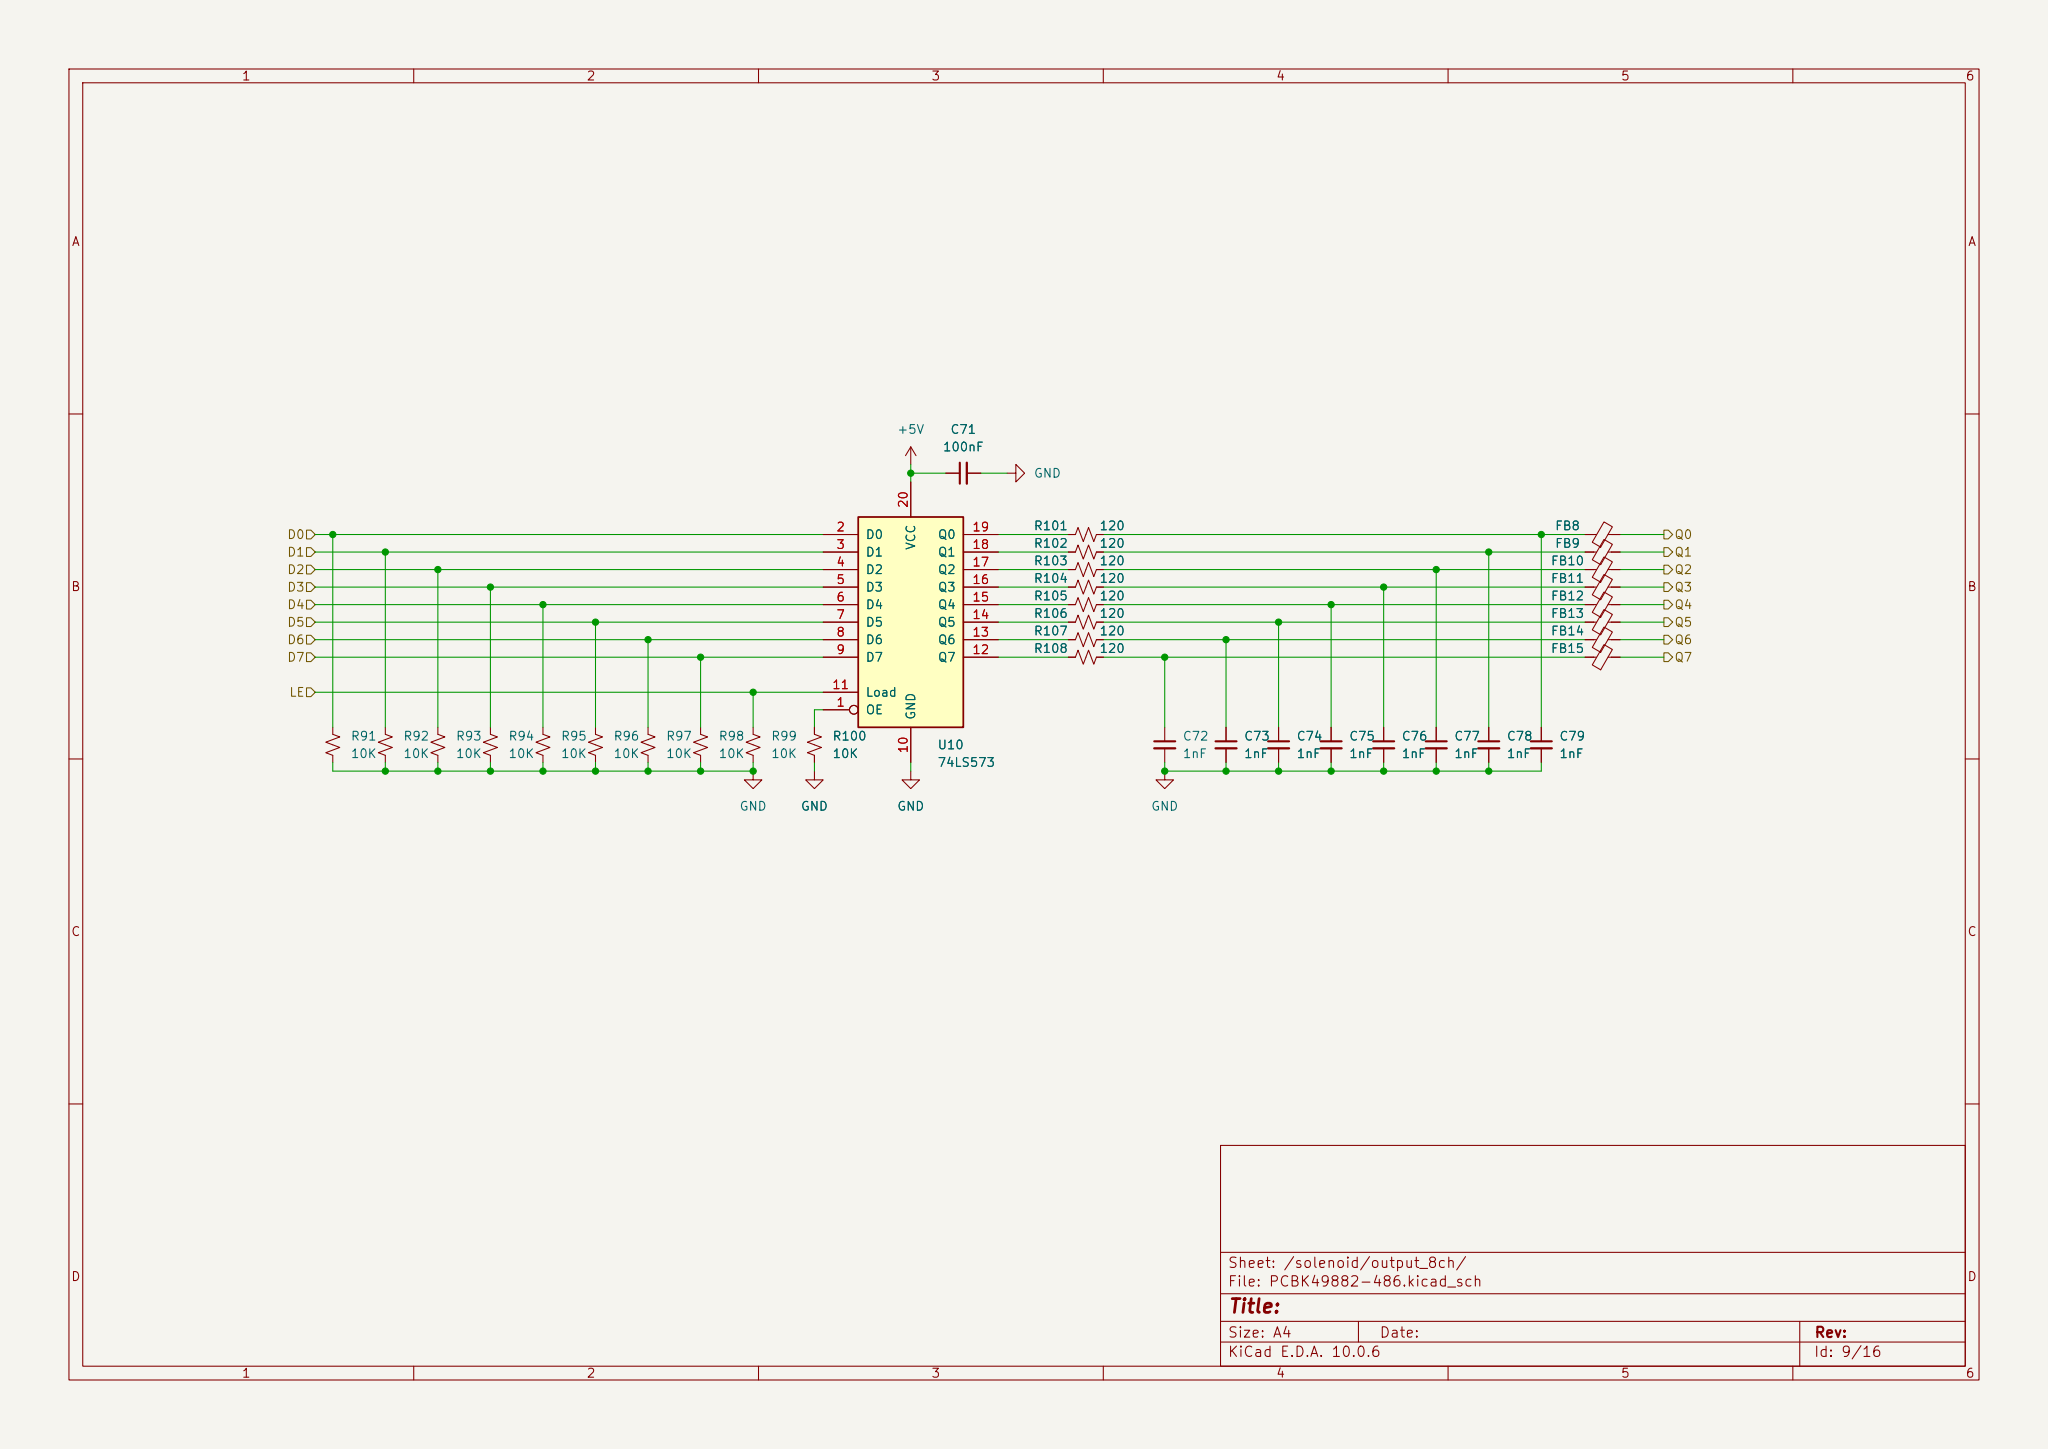Circuit board | KiCad | 536 parts | 438 nets | one sheet of the schematic
Parts on this sheet (reference | value | footprint):
C71
C72
C73
C74
C75
C76
C77
C78
C79
FB10
FB11
FB12
FB13
FB14
FB15
FB8
FB9
R100
R101
R102
R103
R104
R105
R106
R107
R108
R91
R92
R93
R94
R95
R96
R97
R98
R99
U10
Nets of these parts (net: part-pin ...):
+5V: C71-1 U10-20
/core_board_b2b/PA0_C{slash}ADC12_INP0: R91-1 U10-2
/core_board_b2b/PA1_C{slash}ADC12_INP1: R92-1 U10-3
/core_board_b2b/PA3{slash}ADC12_INP15: R95-1 U10-6
/core_board_b2b/PA4{slash}ADC12_INP18: R96-1 U10-7
/core_board_b2b/PA5{slash}ADC12_INP19: R97-1 U10-8
/core_board_b2b/PA6{slash}ADC12_INP3: R98-1 U10-9
/core_board_b2b/PB0{slash}ADC12_INP9: R99-1 U10-11
/core_board_b2b/PC2_C{slash}ADC3_INP0: R93-1 U10-4
/core_board_b2b/PC3_C{slash}ADC3_INP1: R94-1 U10-5
/solenoid/OUTPUT0: FB8-2
/solenoid/OUTPUT1: FB9-2
/solenoid/OUTPUT2: FB10-2
/solenoid/OUTPUT3: FB11-2
/solenoid/OUTPUT4: FB12-2
/solenoid/OUTPUT5: FB13-2
/solenoid/OUTPUT6: FB14-2
/solenoid/OUTPUT7: FB15-2
GND: C71-2 C72-2 C73-2 C74-2 C75-2 C76-2 C77-2 C78-2 C79-2 R91-2 R92-2 R93-2 R94-2 R95-2 R96-2 R97-2 R98-2 R99-2 R100-2 U10-10
Net-(C72-Pad1): C72-1 FB15-1 R108-2
Net-(C73-Pad1): C73-1 FB14-1 R107-2
Net-(C74-Pad1): C74-1 FB13-1 R106-2
Net-(C75-Pad1): C75-1 FB12-1 R105-2
Net-(C76-Pad1): C76-1 FB11-1 R104-2
Net-(C77-Pad1): C77-1 FB10-1 R103-2
Net-(C78-Pad1): C78-1 FB9-1 R102-2
Net-(C79-Pad1): C79-1 FB8-1 R101-2
Net-(U10-OE): R100-1 U10-1
Net-(U10-Q0): R101-1 U10-19
Net-(U10-Q1): R102-1 U10-18
Net-(U10-Q2): R103-1 U10-17
Net-(U10-Q3): R104-1 U10-16
Net-(U10-Q4): R105-1 U10-15
Net-(U10-Q5): R106-1 U10-14
Net-(U10-Q6): R107-1 U10-13
Net-(U10-Q7): R108-1 U10-12